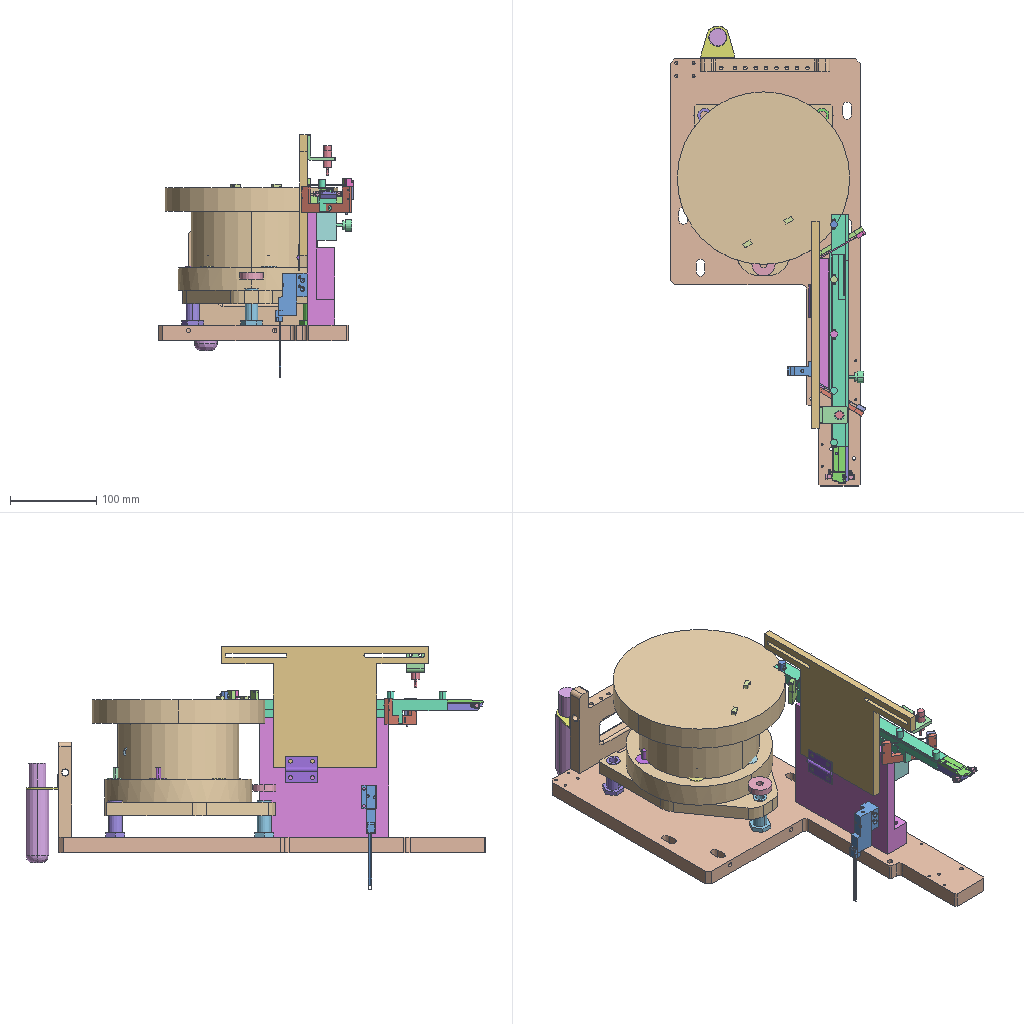Assembly | SolidWorks | 15 different items | 41 placed | box 227 x 533 x 281 mm
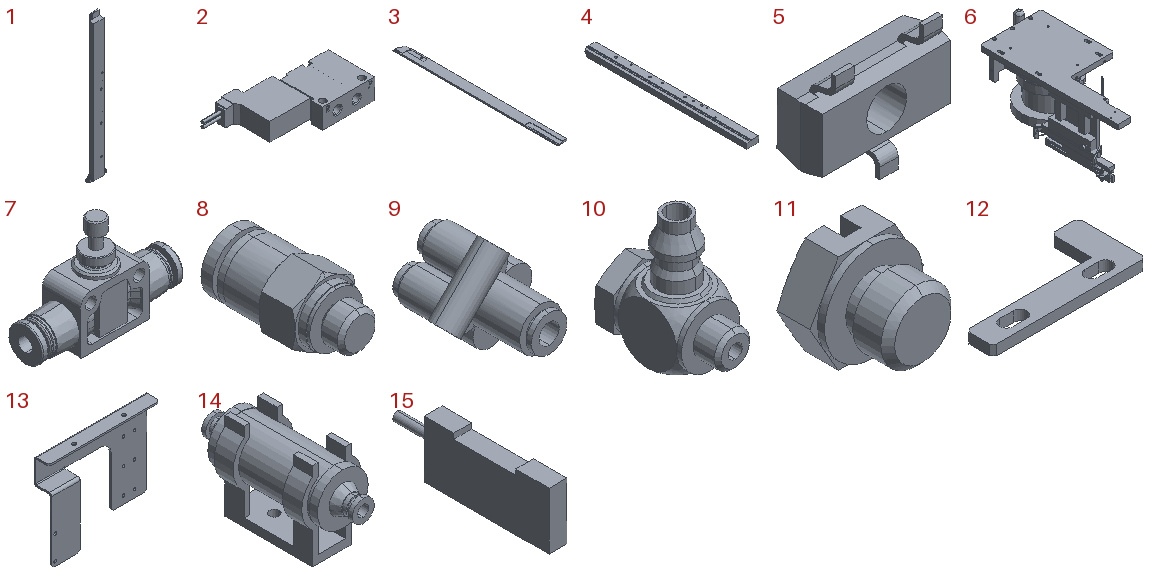Parts list (item | name | quantity | parent item | size | volume | features):
1 | (subassembly) | x1 | - | 33.8 x 12.35 x 265.95 mm | 52246 mm3 | features ReferencePattern 2, LocalLPattern 1
2 | - | x4 | - | 65.3 x 33 x 11 mm | 11908 mm3 | features ICE 2, BaseBody 1
3 | - | x1 | in 1 | 15.5 x 265.95 x 3 mm | 11274 mm3 | features ICE 7, Chamfer 3, Cut 2, Fillet 2, BaseBody 1, HoleWzd 1
4 | - | x1 | in 1 | 19 x 256 x 8.75 mm | 40563 mm3 | features ICE 6, HoleWzd 4, Chamfer 2, BaseBody 1, Cut 1
5 | - | x3 | in 1 | 2.908 x 1.057 x 2.408 mm | 2.992 mm3 | features ICE 6, Fillet 4, Extrusion 1, RefAxis 1
6 | - | x1 | - | 226.504 x 533.25 x 281.45 mm | 5326781 mm3 | features BaseBody 82, ICE 6, HoleWzd 4, Chamfer 2, Cut 1, Fillet 1
7 | - | x4 | - | 40.8 x 11 x 28.611 mm | 4329 mm3 | features BaseBody 1
8 | - | x11 | - | 8 x 17 x 9.238 mm | 564.577 mm3 | features BaseBody 1
9 | - | x2 | - | 29.666 x 35.5 x 29.666 mm | 7119 mm3 | features BaseBody 1
10 | - | x2 | in 1 | 5 x 9.5 x 10.687 mm | 200.167 mm3 | features BaseBody 1
11 | - | x5 | - | 8.083 x 6.5 x 7 mm | 172.442 mm3 | features BaseBody 1
12 | - | x1 | - | 45 x 20 x 3 mm | 1189 mm3 | features Chamfer 1, Extrusion 1, ICE 1
13 | - | x1 | - | 100 x 16 x 79.5 mm | 10218 mm3 | features EdgeFlange 3, HoleWzd 3, Chamfer 1, Fillet 1, FlatPattern 1, ICE 1, LPattern 1, SMBaseFlange 1, SheetMetal 1
14 | - | x3 | - | 22 x 55 x 32 mm | 13292 mm3 | features ICE 3, HoleWzd 2, BaseBody 1
15 | - | x1 | - | 10 x 90 x 32 mm | 21745 mm3 | features BaseBody 1, ICE 1
Mates (type | each side: item.copy, entity, surface, feature):
In the top assembly
Coincident | 6.1 face plane PRT0001_MIR-1-solid1 | 12.1 face plane Boss-Extrude1
Coincident | 6.1 face plane Boss-Extrude1 | 12.1 face plane Boss-Extrude1
DistanceDim | 12.1 face plane Boss-Extrude1 | 6.1 face plane PRT0001_MIR-1-solid1
Coincident | 2.1 face plane Input 1 | 8.1 face plane Input 1
Concentric | 2.1 face cylinder Input 1 | 8.1 face cylinder Input 1
Concentric | 2.1 face cylinder Input 1 | 8.2 face cylinder Input 1
Concentric | 2.1 face cylinder Input 1 | 8.3 face cylinder Input 1
Coincident | 2.1 face plane Input 1 | 8.3 face plane Input 1
Concentric | 2.1 face cylinder Input 1 | 11.1 face cylinder Input 1
Coincident | 2.1 face plane Input 1 | 11.1 face plane Input 1
Coincident | 8.1 face plane Input 1 | 8.2 face plane Input 1
Coincident | 2.1 face plane Input 1 | 13.1 face plane Edge-Flange2 | 3 times
Coincident | 13.1 face plane Base-Flange1 | 14.1 face plane Boss-Extrude1
Coincident | 13.1 face plane Boss-Extrude1 | 14.1 face plane Input 3 | 2 times
Coincident | 6.1 face plane PRT0145_MIR-1-solid1 | 15.1 face plane Input 1 | 3 times
Coincident | 2.2 face plane Input 1 | 2.3 face plane Input 1 | 3 times
Coincident | 2.3 face plane Input 1 | 8.4 face plane Input 1
Concentric | 8.4 face cylinder Input 1 | 2.3 face cylinder Input 1
Concentric | 11.2 face cylinder Input 1 | 2.3 face cylinder Input 1
Coincident | 2.3 face plane Input 1 | 11.2 face plane Input 1
DistanceDim | 13.1 face plane Edge-Flange1 | 6.1 face plane PRT0158_MIR-1-solid1
Coincident | 2.3 face plane Input 1 | 11.3 face plane Input 1
Concentric | 8.5 face cylinder Input 1 | 2.3 face cylinder Input 1
Coincident | 2.3 face plane Input 1 | 8.5 face plane Input 1
Concentric | 2.3 face cylinder Input 1 | 11.3 face cylinder Input 1
Coincident | 9.1 face plane Input 1 | 9.2 face plane Input 1 | 2 times
Concentric | 8.6 face cylinder Input 1 | 9.1 face cylinder Input 1
DistanceDim | 9.1 face plane Input 1 | 8.6 face plane Input 1
Parallel | 2.3 face plane Input 1 | 9.1 face plane Input 1
Concentric | 8.2 face cylinder Input 1 | 7.1 face cylinder Input 1
Concentric | 8.4 face cylinder Input 1 | 7.2 face cylinder Input 1
Parallel | 2.3 face plane Input 1 | 7.1 face plane Input 1
Parallel | 2.3 face plane Input 1 | 7.2 face plane Input 1
Coincident | 6.1 face plane PRT0144_MIR-1-solid1 | 4.1 face plane Input 1
DistanceDim | 5.1 face plane Boss-Extrude1 | 6.1 face plane PRT0001_MIR-1-solid1
DistanceDim | 4.1 face plane Input 1 | 6.1 face plane PRT0001_MIR-1-solid1
Coincident | 6.1 face plane PRT0001_MIR-1-solid1 | 13.1 face plane Edge-Flange3 | 2 times
In subassembly 1
DistanceDim | 4.2 face plane Input 1 | 3.1 face plane Input 1 | 2 times
Coincident | 4.2 face plane Input 1 | 3.1 face plane Input 1
Coincident | 4.2 face plane Input 1 | 10.1 face plane Input 1
Concentric | 4.2 face cylinder M3 Tapped Hole1 | 10.1 face cylinder Input 1
Concentric | 4.2 face cylinder M3 Tapped Hole2 | 10.2 face cylinder Input 1
Coincident | 4.2 face plane Input 1 | 10.2 face plane Input 1
Parallel | 4.2 face plane Input 1 | 10.1 face plane Input 1
Parallel | 10.1 face plane Input 1 | 10.2 face plane Input 1